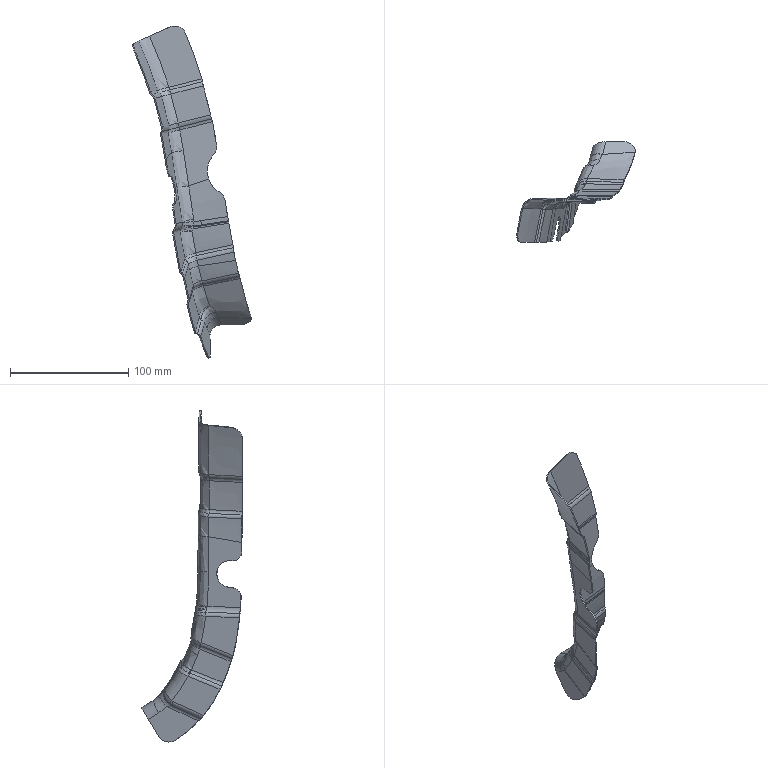Part | STEP file | FNA5401757 | 1 solid | 256 faces | box 100.489 x 85.531 x 281.294 mm | volume 19458 mm3 | spline 221 | cylinder 19 | plane 13 | other 3 | commonest cylinder face diameters 10 x7 8 x5 12 x2 14 x1 16 x1 20 x1